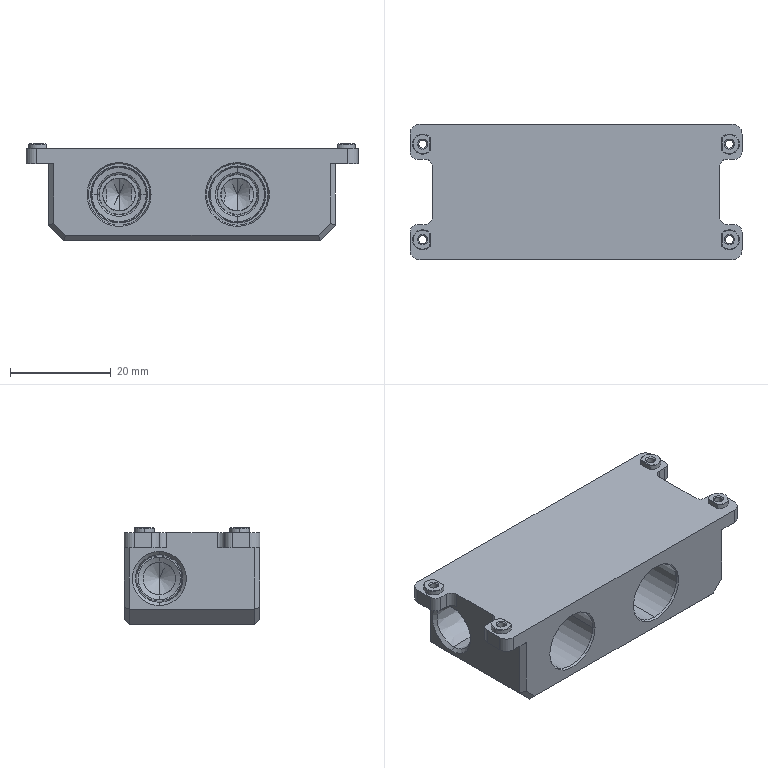NC program | NX | posted with a generic post | part box 66 x 27 x 19.25 mm
Lines 1686 to 2633 of 6448:
(ZLEVEL_PROFILE_STEEP , TOOL : 圆鼻刀)
N3322 T08 M6
N3324 G53
N3326 G17 G0 G90 X-15.95 Y25.719 S6500 M3
N3328 G43 Z20. H8
N3330 Z2.404
N3332 G94 G1 Z1.404 F2000.
N3334 X-15.516 Y25.277
N3336 G3 X-13.819 Y25.262 R1.2
N3338 G2 X-12.468 Y25.803 R1.89
N3340 G1 X12.468
N3342 G2 X13.819 Y25.262 R1.89
N3344 G1 X13.876 Y25.216 Z1.394
N3346 X13.931 Y25.168 Z1.384
N3348 X13.983 Y25.117 Z1.374
N3350 X14.033 Y25.064 Z1.364
N3352 X14.08 Y25.01 Z1.354
N3354 G3 X13.806 Y25.324 R1.983
N3356 G1 X13.759 Y25.367
N3358 G3 X12.496 Y25.853 R1.881
N3360 G1 X-12.509
N3362 G3 X-13.243 Y25.699 R1.818
N3364 X-14.08 Y25.01 R2.008
N3366 G1 X-14.133 Y24.983 Z1.304
N3368 G2 X-13.467 Y25.633 R2.074
N3370 X-12.468 Y25.903 R1.878
N3372 G1 X12.468
N3374 G2 X13.707 Y25.463 R1.896
N3376 X14.133 Y24.983 R2.166
N3378 G1 X14.186 Y24.959 Z1.254
N3380 G3 X13.906 Y25.324 R2.811
N3382 X12.468 Y25.953 R1.909
N3384 G1 X-12.468
N3386 G3 X-13.906 Y25.324 R1.909
N3388 X-14.186 Y24.959 R2.811
N3390 G1 X-14.235 Y24.937 Z1.205
N3392 G2 X-13.951 Y25.324 R4.317
N3394 X-12.468 Y26.003 R1.916
N3396 G1 X12.468
N3398 G2 X13.951 Y25.324 R1.916
N3400 X14.235 Y24.937 R4.318
N3402 G1 X14.286 Y24.916 Z1.155
N3404 X14.017 Y25.294
N3406 X13.964 Y25.358
N3408 G3 X12.485 Y26.052 R1.921
N3410 G1 X-12.485
N3412 G3 X-13.964 Y25.358 R1.921
N3414 G1 X-14.017 Y25.294
N3416 X-14.286 Y24.916
N3418 X-14.337 Y24.895 Z1.105
N3420 X-14.051 Y25.295
N3422 G2 X-12.484 Y26.102 R1.925
N3424 G1 X12.484
N3426 G2 X14.051 Y25.295 R1.925
N3428 G1 X14.337 Y24.895
N3430 X14.387 Y24.874 Z1.055
N3432 X14.052 Y25.344
N3434 G3 X12.485 Y26.152 R1.924
N3436 G1 X-12.485
N3438 G3 X-14.052 Y25.344 R1.924
N3440 G1 X-14.387 Y24.874
N3442 X-14.437 Y24.853 Z1.005
N3444 X-14.052 Y25.394
N3446 G2 X-12.485 Y26.202 R1.923
N3448 G1 X12.485
N3450 G2 X14.052 Y25.394 R1.923
N3452 G1 X14.437 Y24.853
N3454 X14.487 Y24.832 Z0.956
N3456 X14.482 Y24.84
N3458 X14.052 Y25.443
N3460 G3 X12.485 Y26.251 R1.925
N3462 G1 X-12.485
N3464 G3 X-14.052 Y25.443 R1.925
N3466 G1 X-14.482 Y24.84
N3468 X-14.487 Y24.832
N3470 X-14.537 Y24.81 Z0.906
N3472 X-14.503 Y24.86
N3474 X-14.052 Y25.493
N3476 G2 X-12.485 Y26.301 R1.923
N3478 G1 X12.485
N3480 G2 X14.052 Y25.493 R1.923
N3482 G1 X14.503 Y24.86
N3484 X14.537 Y24.81
N3486 X14.587 Y24.789 Z0.856
N3488 X14.538 Y24.86
N3490 X14.053 Y25.542
N3492 G3 X12.485 Y26.351 R1.925
N3494 G1 X-12.485
N3496 G3 X-14.053 Y25.542 R1.925
N3498 G1 X-14.538 Y24.86
N3500 X-14.587 Y24.789
N3502 X-14.638 Y24.768 Z0.806
N3504 G2 X-14.045 Y25.603 R57.54
N3506 X-12.484 Y26.401 R1.927
N3508 G1 X12.484
N3510 G2 X14.045 Y25.603 R1.927
N3512 X14.638 Y24.768 R57.886
N3514 G1 X14.688 Y24.747 Z0.757
N3516 G3 X14.045 Y25.653 R56.973
N3518 X12.483 Y26.451 R1.928
N3520 G1 X-12.483
N3522 G3 X-14.045 Y25.653 R1.928
N3524 X-14.688 Y24.747 R56.616
N3526 G1 X-14.738 Y24.726 Z0.707
N3528 G2 X-14.046 Y25.701 R73.331
N3530 X-12.484 Y26.5 R1.927
N3532 G1 X12.484
N3534 G2 X14.046 Y25.701 R1.927
N3536 X14.738 Y24.725 R73.745
N3538 G1 X14.789 Y24.705 Z0.657
N3540 X14.172 Y25.577
N3542 X14.046 Y25.751
N3544 G3 X12.484 Y26.55 R1.927
N3546 G1 X-12.484
N3548 G3 X-14.046 Y25.751 R1.927
N3550 G1 X-14.172 Y25.577
N3552 X-14.789 Y24.705
N3554 X-14.838 Y24.683 Z0.607
N3556 X-14.824 Y24.705
N3558 X-14.172 Y25.627
N3560 X-14.047 Y25.8
N3562 G2 X-12.483 Y26.6 R1.928
N3564 G1 X12.483
N3566 G2 X14.047 Y25.8 R1.928
N3568 G1 X14.172 Y25.627
N3570 X14.824 Y24.705
N3572 X14.838 Y24.683
N3574 X14.888 Y24.662 Z0.558
N3576 X14.859 Y24.705
N3578 X14.172 Y25.676
N3580 X14.046 Y25.85
N3582 G3 X12.484 Y26.65 R1.927
N3584 G1 X-12.484
N3586 G3 X-14.046 Y25.85 R1.927
N3588 G1 X-14.172 Y25.676
N3590 X-14.859 Y24.705
N3592 X-14.888 Y24.662
N3594 X-14.939 Y24.642 Z0.508
N3596 X-14.894 Y24.705
N3598 X-14.172 Y25.726
N3600 X-14.046 Y25.9
N3602 G2 X-12.484 Y26.699 R1.926
N3604 G1 X12.484
N3606 G2 X14.046 Y25.9 R1.926
N3608 G1 X14.172 Y25.726
N3610 X14.894 Y24.705
N3612 X14.939 Y24.642
N3614 X14.988 Y24.62 Z0.458
N3616 X14.946 Y24.681
N3618 X14.172 Y25.776
N3620 X14.047 Y25.949
N3622 G3 X12.483 Y26.749 R1.929
N3624 G1 X-12.483
N3626 G3 X-14.047 Y25.949 R1.929
N3628 G1 X-14.172 Y25.776
N3630 X-14.946 Y24.681
N3632 X-14.988 Y24.62
N3634 X-15.038 Y24.6 Z0.408
N3636 X-14.964 Y24.705
N3638 X-14.172 Y25.826
N3640 X-14.046 Y26.
N3642 G2 X-12.484 Y26.799 R1.926
N3644 G1 X12.484
N3646 G2 X14.046 Y25.999 R1.926
N3648 G1 X14.172 Y25.826
N3650 X14.964 Y24.705
N3652 X15.038 Y24.6
N3654 X15.088 Y24.579 Z0.358
N3656 X14.172 Y25.875
N3658 X14.042 Y26.055
N3660 G3 X12.486 Y26.849 R1.92
N3662 G1 X-12.486
N3664 G3 X-14.041 Y26.055 R1.92
N3666 G1 X-14.172 Y25.875
N3668 X-15.088 Y24.579
N3670 X-15.138 Y24.559 Z0.309
N3672 X-14.172 Y25.925
N3674 X-14.047 Y26.098
N3676 G2 X-12.483 Y26.898 R1.929
N3678 G1 X12.483
N3680 G2 X14.047 Y26.098 R1.929
N3682 G1 X14.172 Y25.925
N3684 X15.138 Y24.559
N3686 X15.188 Y24.538 Z0.259
N3688 X15.179 Y24.551
N3690 X14.172 Y25.975
N3692 X14.046 Y26.149
N3694 G3 X12.484 Y26.948 R1.926
N3696 G1 X-12.484
N3698 G3 X-14.046 Y26.149 R1.926
N3700 G1 X-14.172 Y25.975
N3702 X-15.179 Y24.551
N3704 X-15.188 Y24.538
N3706 X-15.237 Y24.518 Z0.209
N3708 X-14.172 Y26.025
N3710 X-14.039 Y26.208
N3712 G2 X-12.487 Y26.998 R1.919
N3714 G1 X12.487
N3716 G2 X14.039 Y26.208 R1.919
N3718 G1 X14.172 Y26.025
N3720 X15.237 Y24.518
N3722 X15.286 Y24.497 Z0.159
N3724 X15.256 Y24.542
N3726 X14.172 Y26.074
N3728 X14.046 Y26.249
N3730 G3 X12.485 Y27.048 R1.924
N3732 G1 X-12.485
N3734 G3 X-14.046 Y26.249 R1.924
N3736 G1 X-14.172 Y26.074
N3738 X-15.256 Y24.542
N3740 X-15.286 Y24.497
N3742 X-15.336 Y24.476 Z0.11
N3744 X-15.285 Y24.551
N3746 X-14.172 Y26.124
N3748 X-14.046 Y26.298
N3750 G2 X-12.484 Y27.098 R1.926
N3752 G1 X12.484
N3754 G2 X14.046 Y26.298 R1.926
N3756 G1 X14.172 Y26.124
N3758 X15.285 Y24.551
N3760 X15.336 Y24.476
N3762 X15.386 Y24.456 Z0.06
N3764 X15.32 Y24.551
N3766 X14.172 Y26.174
N3768 X14.047 Y26.347
N3770 G3 X12.483 Y27.147 R1.928
N3772 G1 X-12.483
N3774 G3 X-14.047 Y26.347 R1.928
N3776 G1 X-14.172 Y26.174
N3778 X-15.32 Y24.551
N3780 X-15.386 Y24.456
N3782 X-15.436 Y24.436 Z0.01
N3784 X-15.411 Y24.472
N3786 X-14.172 Y26.224
N3788 X-14.046 Y26.398
N3790 G2 X-12.485 Y27.197 R1.925
N3792 G1 X12.485
N3794 G2 X14.046 Y26.398 R1.925
N3796 G1 X14.172 Y26.224
N3798 X15.411 Y24.472
N3800 X15.436 Y24.436
N3802 X15.485 Y24.416 Z-0.04
N3804 X15.411 Y24.522
N3806 X14.172 Y26.273
N3808 X14.047 Y26.447
N3810 G3 X12.484 Y27.247 R1.927
N3812 G1 X-12.484
N3814 G3 X-14.047 Y26.447 R1.927
N3816 G1 X-14.172 Y26.274
N3818 X-15.411 Y24.522
N3820 X-15.485 Y24.416
N3822 X-15.535 Y24.396 Z-0.09
N3824 X-14.172 Y26.323
N3826 X-14.047 Y26.496
N3828 G2 X-12.483 Y27.297 R1.928
N3830 G1 X12.483
N3832 G2 X14.047 Y26.496 R1.928
N3834 G1 X14.172 Y26.323
N3836 X15.535 Y24.396
N3838 X15.584 Y24.375 Z-0.139
N3840 X15.57 Y24.396
N3842 X14.172 Y26.373
N3844 X14.046 Y26.547
N3846 G3 X12.484 Y27.346 R1.926
N3848 G1 X-12.484
N3850 G3 X-14.046 Y26.547 R1.926
N3852 G1 X-14.172 Y26.373
N3854 X-15.57 Y24.396
N3856 X-15.584 Y24.375
N3858 X-15.633 Y24.355 Z-0.189
N3860 X-15.606 Y24.396
N3862 X-14.172 Y26.423
N3864 X-14.017 Y26.638
N3866 G2 X-12.5 Y27.396 R1.932
N3868 G1 X12.5
N3870 G2 X14.017 Y26.638 R1.932
N3872 G1 X14.172 Y26.423
N3874 X15.606 Y24.396
N3876 X15.634 Y24.355
N3878 X15.683 Y24.334 Z-0.239
N3880 X15.641 Y24.396
N3882 X14.172 Y26.473
N3884 X14.017 Y26.687
N3886 G3 X12.5 Y27.446 R1.928
N3888 G1 X-12.5
N3890 G3 X-14.017 Y26.687 R1.928
N3892 G1 X-14.172 Y26.473
N3894 X-15.641 Y24.396
N3896 X-15.683 Y24.334
N3898 X-15.733 Y24.314 Z-0.289
N3900 X-15.721 Y24.333
N3902 X-14.172 Y26.522
N3904 X-14.034 Y26.716
N3906 G2 X-12.5 Y27.496 R1.933
N3908 G1 X12.5
N3910 G2 X14.034 Y26.716 R1.933
N3912 G1 X14.172 Y26.522
N3914 X15.721 Y24.333
N3916 X15.733 Y24.314
N3918 X15.782 Y24.294 Z-0.338
N3920 X15.721 Y24.383
N3922 X14.07 Y26.716
N3924 G3 X12.5 Y27.545 R1.941
N3926 G1 X-12.5
N3928 G3 X-14.07 Y26.716 R1.941
N3930 G1 X-15.721 Y24.383
N3932 X-15.782 Y24.294
N3934 X-15.832 Y24.274 Z-0.388
N3936 X-15.747 Y24.396
N3938 X-14.216 Y26.559
N3940 X-14.078 Y26.754
N3942 G2 X-12.5 Y27.595 R1.945
N3944 G1 X12.5
N3946 G2 X14.078 Y26.754 R1.945
N3948 G1 X14.216 Y26.559
N3950 X15.747 Y24.396
N3952 X15.832 Y24.274
N3954 X15.882 Y24.254 Z-0.438
N3956 X14.266 Y26.538
N3958 X14.078 Y26.804
N3960 G3 X12.5 Y27.645 R1.945
N3962 G1 X-12.5
N3964 G3 X-14.078 Y26.804 R1.945
N3966 G1 X-14.266 Y26.538
N3968 X-15.882 Y24.254
N3970 X-15.932 Y24.233 Z-0.488
N3972 X-14.316 Y26.518
N3974 X-14.078 Y26.854
N3976 G2 X-12.5 Y27.695 R1.945
N3978 G1 X12.5
N3980 G2 X14.078 Y26.854 R1.945
N3982 G1 X14.316 Y26.518
N3984 X15.932 Y24.233
N3986 X15.981 Y24.213 Z-0.537
N3988 X15.962 Y24.241
N3990 X14.366 Y26.497
N3992 X14.078 Y26.904
N3994 G3 X13.845 Y27.179 R2.184
N3996 X12.5 Y27.745 R1.904
N3998 G1 X-12.512
N4000 G3 X-13.088 Y27.649 R1.786
N4002 X-14.078 Y26.904 R1.989
N4004 G1 X-14.366 Y26.497
N4006 X-15.962 Y24.241
N4008 X-15.981 Y24.213
N4010 X-16.031 Y24.193 Z-0.587
N4012 X-14.416 Y26.476
N4014 X-14.078 Y26.953
N4016 G2 X-13.088 Y27.699 R1.988
N4018 X-12.512 Y27.794 R1.787
N4020 G1 X12.5
N4022 G2 X13.321 Y27.602 R1.846
N4024 X14.078 Y26.953 R2.036
N4026 G1 X14.416 Y26.476
N4028 X16.031 Y24.193
N4030 X16.08 Y24.172 Z-0.637
N4032 X16.032 Y24.241
N4034 X14.465 Y26.456
N4036 X14.078 Y27.003
N4038 G3 X12.5 Y27.844 R1.945
N4040 G1 X-12.5
N4042 G3 X-14.078 Y27.003 R1.945
N4044 G1 X-14.465 Y26.456
N4046 X-16.032 Y24.241
N4048 X-16.08 Y24.172
N4050 X-16.13 Y24.152 Z-0.687
N4052 X-16.067 Y24.241
N4054 X-14.515 Y26.435
N4056 X-14.078 Y27.053
N4058 G2 X-13.088 Y27.799 R1.989
N4060 X-12.512 Y27.894 R1.786
N4062 G1 X12.5
N4064 G2 X13.702 Y27.459 R1.878
N4066 X14.078 Y27.053 R2.16
N4068 G1 X14.515 Y26.435
N4070 X16.067 Y24.241
N4072 X16.13 Y24.152
N4074 X16.18 Y24.132 Z-0.737
N4076 X14.565 Y26.414
N4078 X14.078 Y27.103
N4080 G3 X13.295 Y27.764 R2.03
N4082 X12.5 Y27.944 R1.844
N4084 G1 X-12.512
N4086 G3 X-13.088 Y27.848 R1.788
N4088 X-14.078 Y27.103 R1.988
N4090 G1 X-14.565 Y26.414
N4092 X-16.18 Y24.132
N4094 X-16.229 Y24.111 Z-0.786
N4096 X-16.185 Y24.174
N4098 X-14.615 Y26.394
N4100 X-14.078 Y27.152
N4102 G2 X-12.5 Y27.993 R1.945
N4104 G1 X12.5
N4106 G2 X14.078 Y27.152 R1.945
N4108 G1 X14.615 Y26.394
N4110 X16.185 Y24.174
N4112 X16.229 Y24.111
N4114 X16.279 Y24.091 Z-0.836
N4116 X14.664 Y26.373
N4118 X14.078 Y27.202
N4120 G3 X13.672 Y27.632 R2.138
N4122 X12.5 Y28.043 R1.876
N4124 G1 X-12.509
N4126 G3 X-13.243 Y27.889 R1.819
N4128 X-14.078 Y27.202 R2.009
N4130 G1 X-14.664 Y26.373
N4132 X-16.279 Y24.091
N4134 X-16.328 Y24.071 Z-0.886
N4136 X-16.318 Y24.087
N4138 X-14.714 Y26.353
N4140 X-14.078 Y27.252
N4142 G2 X-13.088 Y27.998 R1.987
N4144 X-12.511 Y28.093 R1.789
N4146 G1 X12.5
N4148 G2 X13.718 Y27.643 R1.893
N4150 X14.078 Y27.252 R2.079
N4152 G1 X14.714 Y26.353
N4154 X16.328 Y24.071
N4156 X16.377 Y24.05 Z-0.936
N4158 X16.353 Y24.087
N4160 X14.764 Y26.332
N4162 X14.078 Y27.302
N4164 G3 X12.5 Y28.143 R1.945
N4166 G1 X-12.5
N4168 G3 X-14.078 Y27.302 R1.945
N4170 G1 X-14.764 Y26.332
N4172 X-16.353 Y24.087
N4174 X-16.377 Y24.05
N4176 X-16.427 Y24.03 Z-0.985
N4178 X-16.388 Y24.087
N4180 X-14.814 Y26.311
N4182 X-14.078 Y27.351
N4184 G2 X-13.243 Y28.038 R2.009
N4186 X-12.509 Y28.193 R1.82
N4188 G1 X12.5
N4190 G2 X13.642 Y27.805 R1.874
N4192 X14.078 Y27.351 R2.119
N4194 G1 X14.814 Y26.311
N4196 X16.388 Y24.087
N4198 X16.427 Y24.03
N4200 X16.477 Y24.01 Z-1.035
N4202 X16.423 Y24.087
N4204 X14.863 Y26.291
N4206 X14.078 Y27.401
N4208 G3 X13.578 Y27.901 R2.084
N4210 X12.5 Y28.242 R1.87
N4212 G1 X-12.511
N4214 G3 X-13.088 Y28.147 R1.79
N4216 X-14.078 Y27.401 R1.986
N4218 G1 X-14.863 Y26.291
N4220 X-16.423 Y24.087
N4222 X-16.477 Y24.01
N4224 X-16.51 Y24.013 Z-1.085
N4226 X-16.495 Y24.035
N4228 X-14.913 Y26.27
N4230 X-14.078 Y27.451
N4232 G2 X-13.088 Y28.197 R1.987
N4234 X-12.511 Y28.292 R1.789
N4236 G1 X12.5
N4238 G2 X13.862 Y27.71 R1.909
N4240 X14.078 Y27.451 R2.225
N4242 G1 X14.913 Y26.27
N4244 X16.495 Y24.035
N4246 X16.51 Y24.013
N4248 X16.523 Y24.021 Z-1.11
N4250 X16.535 Y24.028 Z-1.135
N4252 X16.495 Y24.085
N4254 X14.953 Y26.264
N4256 X14.078 Y27.501
N4258 G3 X13.613 Y27.975 R2.104
N4260 X12.5 Y28.342 R1.872
N4262 G1 X-12.512
N4264 G3 X-13.088 Y28.246 R1.787
N4266 X-14.078 Y27.501 R1.988
N4268 G1 X-14.953 Y26.264
N4270 X-16.495 Y24.085
N4272 X-16.535 Y24.028
N4274 X-16.547 Y24.036 Z-1.16
N4276 X-16.559 Y24.044 Z-1.185
N4278 X-14.973 Y26.286
N4280 X-14.078 Y27.551
N4282 G2 X-13.088 Y28.296 R1.986
N4284 X-12.511 Y28.392 R1.792
N4286 G1 X12.5
N4288 G2 X13.699 Y27.96 R1.878
N4290 X14.078 Y27.551 R2.143
N4292 G1 X14.973 Y26.286
N4294 X16.559 Y24.044
N4296 X16.571 Y24.051 Z-1.209
N4298 X16.584 Y24.059 Z-1.234
N4300 X14.992 Y26.308
N4302 X14.078 Y27.6
N4304 G3 X13.862 Y27.859 R2.25
N4306 X12.5 Y28.441 R1.909
N4308 G1 X-12.511
N4310 G3 X-13.088 Y28.346 R1.788
N4312 X-14.078 Y27.6 R1.988
N4314 G1 X-14.992 Y26.308
N4316 X-16.583 Y24.059
N4318 X-16.596 Y24.067 Z-1.259
N4320 X-16.608 Y24.075 Z-1.284
N4322 X-15.012 Y26.33
N4324 X-14.078 Y27.65
N4326 G2 X-13.088 Y28.396 R1.987
N4328 X-12.511 Y28.491 R1.789
N4330 G1 X12.5
N4332 G2 X13.591 Y28.14 R1.871
N4334 X14.078 Y27.65 R2.092
N4336 G1 X15.012 Y26.33
N4338 X16.608 Y24.075
N4340 X16.627 Y24.097 Z-1.334
N4342 X15.078 Y26.286
N4344 X14.078 Y27.7
N4346 G3 X12.5 Y28.541 R1.945
N4348 G1 X-12.5
N4350 G3 X-14.078 Y27.7 R1.945
N4352 G1 X-15.078 Y26.286
N4354 X-16.627 Y24.097
N4356 Y24.147 Z-1.384
N4358 X-16.56 Y24.241
N4360 X-15.078 Y26.335
N4362 X-14.078 Y27.75
N4364 G2 X-13.088 Y28.495 R1.988
N4366 X-12.511 Y28.591 R1.788
N4368 G1 X12.5
N4370 G2 X13.482 Y28.311 R1.861
N4372 X14.078 Y27.75 R2.068
N4374 G1 X15.078 Y26.335
N4376 X16.56 Y24.241
N4378 X16.627 Y24.147
N4380 Y24.196 Z-1.433
N4382 X16.596 Y24.241
N4384 X15.078 Y26.385
N4386 X14.078 Y27.799
N4388 G3 X13.574 Y28.302 R2.083
N4390 X12.5 Y28.64 R1.871
N4392 G1 X-12.511
N4394 G3 X-13.088 Y28.545 R1.79
N4396 X-14.078 Y27.799 R1.987
N4398 G1 X-15.078 Y26.385
N4400 X-16.596 Y24.241
N4402 X-16.627 Y24.196
N4404 Y24.246 Z-1.483
N4406 X-15.078 Y26.435
N4408 X-14.078 Y27.849
N4410 G2 X-12.5 Y28.69 R1.945
N4412 G1 X12.5
N4414 G2 X14.078 Y27.849 R1.945
N4416 G1 X15.078 Y26.435
N4418 X16.628 Y24.246
N4420 Y24.295 Z-1.533
N4422 X16.557 Y24.396
N4424 X15.078 Y26.485
N4426 X14.078 Y27.899
N4428 G3 X13.438 Y28.486 R2.059
N4430 X12.5 Y28.74 R1.857
N4432 G1 X-12.511
N4434 G3 X-13.088 Y28.645 R1.789
N4436 X-14.078 Y27.899 R1.987
N4438 G1 X-15.078 Y26.485
N4440 X-16.557 Y24.396
N4442 X-16.627 Y24.295
N4444 X-16.628 Y24.345 Z-1.583
N4446 X-16.592 Y24.396
N4448 X-15.078 Y26.534
N4450 X-14.078 Y27.949
N4452 G2 X-13.088 Y28.694 R1.987
N4454 X-12.511 Y28.79 R1.789
N4456 G1 X12.5
N4458 G2 X13.862 Y28.208 R1.909
N4460 X14.078 Y27.949 R2.206
N4462 G1 X15.078 Y26.534
N4464 X16.592 Y24.396
N4466 X16.628 Y24.345
N4468 Y24.394 Z-1.632
N4470 X15.078 Y26.584
N4472 X14.078 Y27.998
N4474 G3 X12.5 Y28.84 R1.945
N4476 G1 X-12.5
N4478 G3 X-14.078 Y27.998 R1.945
N4480 G1 X-15.078 Y26.584
N4482 X-16.628 Y24.394
N4484 Y24.444 Z-1.682
N4486 X-16.553 Y24.551
N4488 X-15.078 Y26.634
N4490 X-14.078 Y28.048
N4492 G2 X-13.088 Y28.794 R1.988
N4494 X-12.512 Y28.889 R1.787
N4496 G1 X12.5
N4498 G2 X13.862 Y28.307 R1.909
N4500 G1 X13.904 Y28.262
N4502 G2 X14.078 Y28.048 R2.051
N4504 G1 X15.078 Y26.634
N4506 X16.553 Y24.551
N4508 X16.628 Y24.444
N4510 Y24.493 Z-1.732
N4512 X16.588 Y24.551
N4514 X15.078 Y26.684
N4516 X14.078 Y28.098
N4518 G3 X13.862 Y28.357 R2.179
N4520 X12.5 Y28.939 R1.909
N4522 G1 X-12.511
N4524 G3 X-13.088 Y28.844 R1.789
N4526 X-14.078 Y28.098 R1.987
N4528 G1 X-15.078 Y26.684
N4530 X-16.588 Y24.551
N4532 X-16.628 Y24.493
N4534 X-16.629 Y24.543 Z-1.782
N4536 X-15.078 Y26.734
N4538 X-14.078 Y28.148
N4540 G2 X-13.088 Y28.894 R1.988
N4542 X-12.511 Y28.989 R1.788
N4544 G1 X12.5
N4546 G2 X13.852 Y28.417 R1.906
N4548 X14.078 Y28.148 R2.218
N4550 G1 X15.078 Y26.734
N4552 X16.629 Y24.543
N4554 Y24.592 Z-1.832
N4556 X16.549 Y24.705
N4558 X15.078 Y26.783
N4560 X14.078 Y28.198
N4562 G3 X13.361 Y28.826 R2.044
N4564 X12.5 Y29.039 R1.849
N4566 G1 X-12.512
N4568 G3 X-13.088 Y28.943 R1.787
N4570 X-14.078 Y28.198 R1.988
N4572 G1 X-15.078 Y26.783
N4574 X-16.549 Y24.705
N4576 X-16.629 Y24.592
N4578 Y24.642 Z-1.881
N4580 X-16.584 Y24.705
N4582 X-15.078 Y26.833
N4584 X-14.078 Y28.247
N4586 G2 X-12.5 Y29.088 R1.945
N4588 G1 X12.5
N4590 G2 X14.078 Y28.247 R1.945
N4592 G1 X15.078 Y26.833
N4594 X16.584 Y24.705
N4596 X16.629 Y24.642
N4598 Y24.691 Z-1.931
N4600 X15.078 Y26.883
N4602 X14.078 Y28.297
N4604 G3 X13.847 Y28.571 R2.193
N4606 X12.5 Y29.138 R1.904
N4608 G1 X-12.512
N4610 G3 X-13.088 Y29.043 R1.787
N4612 X-14.078 Y28.297 R1.989
N4614 G1 X-15.078 Y26.883
N4616 X-16.629 Y24.691
N4618 Y24.741 Z-1.981
N4620 X-16.545 Y24.86
N4622 X-15.078 Y26.933
N4624 X-14.078 Y28.347
N4626 G2 X-13.088 Y29.093 R1.988
N4628 X-12.512 Y29.188 R1.787
N4630 G1 X12.5
N4632 G2 X13.33 Y28.991 R1.846
N4634 X14.078 Y28.347 R2.038
N4636 G1 X15.078 Y26.933
N4638 X16.545 Y24.86
N4640 X16.629 Y24.741
N4642 Y24.79 Z-2.031
N4644 X15.078 Y26.982
N4646 X14.078 Y28.397
N4648 G3 X12.5 Y29.238 R1.945
N4650 G1 X-12.5
N4652 G3 X-14.078 Y28.397 R1.945
N4654 G1 X-15.078 Y26.982
N4656 X-16.629 Y24.79
N4658 X-16.63 Y24.84 Z-2.08
N4660 X-15.078 Y27.032
N4662 X-14.078 Y28.446
N4664 G2 X-13.088 Y29.192 R1.989
N4666 X-12.512 Y29.288 R1.786
N4668 G1 X12.5
N4670 G2 X13.712 Y28.844 R1.878
N4672 X14.078 Y28.446 R2.168
N4674 G1 X15.078 Y27.032
N4676 X16.63 Y24.84
N4678 Y24.889 Z-2.13
N4680 X16.542 Y25.015
N4682 X15.078 Y27.082
N4684 X14.078 Y28.496
N4686 G3 X13.302 Y29.154 R2.032
N4688 X12.5 Y29.337 R1.844
N4690 G1 X-12.512
N4692 G3 X-13.088 Y29.242 R1.787
N4694 X-14.078 Y28.496 R1.988
N4696 G1 X-15.078 Y27.082
N4698 X-16.542 Y25.015
N4700 X-16.63 Y24.889
N4702 Y24.939 Z-2.18
N4704 X-15.078 Y27.132
N4706 X-14.078 Y28.546
N4708 G2 X-12.5 Y29.387 R1.945
N4710 G1 X12.5
N4712 G2 X14.078 Y28.546 R1.945
N4714 G1 X15.078 Y27.132
N4716 X16.63 Y24.939
N4718 Y24.988 Z-2.23
N4720 X15.078 Y27.182
N4722 X14.078 Y28.596
N4724 G3 X13.683 Y29.017 R2.145
N4726 X12.5 Y29.437 R1.876
N4728 G1 X-12.512
N4730 G3 X-13.088 Y29.341 R1.786
N4732 X-14.078 Y28.596 R1.989
N4734 G1 X-15.078 Y27.182
N4736 X-16.63 Y24.988
N4738 Y25.038 Z-2.279
N4740 X-15.078 Y27.231
N4742 X-14.078 Y28.646
N4744 G2 X-13.088 Y29.391 R1.988
N4746 X-12.511 Y29.487 R1.788
N4748 G1 X12.5
N4750 G2 X13.279 Y29.314 R1.842
N4752 X14.078 Y28.646 R2.027
N4754 G1 X15.078 Y27.231
N4756 X16.63 Y25.038
N4758 X16.631 Y25.087 Z-2.329
N4760 X15.078 Y27.281
N4762 X14.078 Y28.695
N4764 G3 X12.5 Y29.536 R1.945
N4766 G1 X-12.5
N4768 G3 X-14.078 Y28.695 R1.945
N4770 G1 X-15.078 Y27.281
N4772 X-16.631 Y25.087
N4774 Y25.137 Z-2.379
N4776 X-15.078 Y27.331
N4778 X-14.078 Y28.745
N4780 G2 X-13.243 Y29.432 R2.009
N4782 X-12.509 Y29.586 R1.82
N4784 G1 X12.5
N4786 G2 X13.707 Y29.146 R1.895
N4788 G1 X13.79 Y29.071
N4790 G2 X14.074 Y28.751 R1.952
N4792 G1 X15.078 Y27.331
N4794 X16.631 Y25.137
N4796 Y25.186 Z-2.429
N4798 X15.078 Y27.381
N4800 X14.078 Y28.795
N4802 G3 X13.502 Y29.344 R2.063
N4804 X12.5 Y29.636 R1.865
N4806 G1 X-12.511
N4808 G3 X-13.088 Y29.541 R1.79
N4810 X-14.078 Y28.795 R1.987
N4812 G1 X-15.078 Y27.381
N4814 X-16.631 Y25.187
N4816 Y25.236 Z-2.479
N4818 X-15.078 Y27.43
N4820 X-14.078 Y28.845
N4822 G2 X-12.5 Y29.686 R1.945
N4824 G1 X12.5
N4826 G2 X14.078 Y28.845 R1.945
N4828 G1 X15.078 Y27.43
N4830 X16.631 Y25.236
N4832 Y25.285 Z-2.528
N4834 X15.078 Y27.48
N4836 X14.078 Y28.894
N4838 G3 X13.624 Y29.361 R2.109
N4840 X12.5 Y29.735 R1.873
N4842 G1 X-12.512
N4844 G3 X-13.088 Y29.64 R1.787
N4846 X-14.078 Y28.894 R1.989
N4848 G1 X-15.078 Y27.48
N4850 X-16.631 Y25.286
N4852 X-16.632 Y25.335 Z-2.578
N4854 X-15.078 Y27.53
N4856 X-14.078 Y28.944
N4858 G2 X-13.088 Y29.69 R1.986
N4860 X-12.511 Y29.785 R1.792
N4862 G1 X12.5
N4864 G2 X13.666 Y29.379 R1.876
N4866 X14.078 Y28.944 R2.123
N4868 G1 X15.078 Y27.53
N4870 X16.632 Y25.335
N4872 Y25.384 Z-2.628
N4874 X15.078 Y27.58
N4876 X14.078 Y28.994
N4878 G3 X13.862 Y29.253 R2.242
N4880 X12.5 Y29.835 R1.909
N4882 G1 X-12.511
N4884 G3 X-13.088 Y29.74 R1.788
N4886 X-14.078 Y28.994 R1.988
N4888 G1 X-15.078 Y27.58
N4890 X-16.632 Y25.384
N4892 Y25.434 Z-2.678
N4894 X-15.078 Y27.629
N4896 X-14.078 Y29.044
N4898 G2 X-13.088 Y29.789 R1.988
N4900 X-12.511 Y29.885 R1.788
N4902 G1 X12.5
N4904 G2 X13.597 Y29.53 R1.871
N4906 X14.078 Y29.044 R2.096
N4908 G1 X15.078 Y27.629
N4910 X16.632 Y25.434
N4912 Y25.484 Z-2.727
N4914 X15.078 Y27.679
N4916 X14.078 Y29.093
N4918 G3 X12.5 Y29.935 R1.945
N4920 G1 X-12.5
N4922 G3 X-14.078 Y29.093 R1.945
N4924 G1 X-15.078 Y27.679
N4926 X-16.632 Y25.484
N4928 Y25.533 Z-2.777
N4930 X-15.078 Y27.729
N4932 X-14.078 Y29.143
N4934 G2 X-13.088 Y29.889 R1.988
N4936 X-12.511 Y29.984 R1.788
N4938 G1 X12.5
N4940 G2 X13.862 Y29.402 R1.909
N4942 X14.078 Y29.143 R2.261
N4944 G1 X15.078 Y27.729
N4946 X16.632 Y25.533
N4948 Y25.583 Z-2.827
N4950 X15.078 Y27.779
N4952 X14.078 Y29.193
N4954 G3 X13.579 Y29.692 R2.086
N4956 X12.5 Y30.034 R1.871
N4958 G1 X-12.511
N4960 G3 X-13.088 Y29.939 R1.789
N4962 X-14.078 Y29.193 R1.987
N4964 G1 X-15.078 Y27.779
N4966 X-16.632 Y25.583
N4968 X-16.633 Y25.632 Z-2.877
N4970 X-15.078 Y27.829
N4972 X-14.078 Y29.243
N4974 G2 X-12.5 Y30.084 R1.945
N4976 G1 X12.5
N4978 G2 X14.078 Y29.243 R1.945
N4980 G1 X15.078 Y27.829
N4982 X16.633 Y25.632
N4984 Y25.682 Z-2.927
N4986 X15.078 Y27.878
N4988 X14.078 Y29.293
N4990 G3 X13.453 Y29.871 R2.062
N4992 X12.5 Y30.134 R1.858
N4994 G1 X-12.511
N4996 G3 X-13.088 Y30.038 R1.789
N4998 X-14.078 Y29.293 R1.987
N5000 G1 X-15.078 Y27.878
N5002 X-16.633 Y25.682
N5004 Y25.731 Z-2.976
N5006 X-15.078 Y27.928
N5008 X-14.078 Y29.342
N5010 G2 X-13.088 Y30.088 R1.988
N5012 X-12.512 Y30.183 R1.788
N5014 G1 X12.5
N5016 G2 X13.565 Y29.85 R1.87
N5018 X14.078 Y29.342 R2.078
N5020 G1 X15.078 Y27.928
N5022 X16.633 Y25.731
N5024 Y25.781 Z-3.026
N5026 X15.078 Y27.978
N5028 X14.078 Y29.392
N5030 G3 X12.5 Y30.233 R1.945
N5032 G1 X-12.5
N5034 G3 X-14.078 Y29.392 R1.945
N5036 G1 X-15.078 Y27.978
N5038 X-16.633 Y25.781
N5040 Y25.831 Z-3.076
N5042 X-15.078 Y28.028
N5044 X-14.078 Y29.442
N5046 G2 X-13.088 Y30.188 R1.991
N5048 X-12.512 Y30.283 R1.783
N5050 G1 X12.5
N5052 G2 X13.395 Y30.052 R1.853
N5054 X14.078 Y29.442 R2.051
N5056 G1 X15.078 Y28.028
N5058 X16.633 Y25.831
N5060 Y25.88 Z-3.126
N5062 X15.078 Y28.077
N5064 X14.078 Y29.492
N5066 G3 X13.836 Y29.777 R2.147
N5068 X12.479 Y30.333 R1.932
N5070 G1 X-12.514
N5072 G3 X-12.933 Y30.282 R1.739
N5074 X-14.078 Y29.492 R1.972
N5076 G1 X-15.078 Y28.077
N5078 X-16.633 Y25.88
N5080 Y25.93 Z-3.175
N5082 X-15.078 Y28.127
N5084 X-14.078 Y29.541
N5086 G2 X-13.088 Y30.287 R1.986
N5088 X-12.511 Y30.382 R1.791
N5090 G1 X12.481
N5092 G2 X13.862 Y29.801 R1.909
N5094 X14.078 Y29.541 R2.327
N5096 G1 X15.078 Y28.127
N5098 X16.633 Y25.93
N5100 Y25.979 Z-3.225
N5102 X15.078 Y28.177
N5104 X14.078 Y29.591
N5106 G3 X13.901 Y29.808 R2.015
N5108 G1 X13.887 Y29.823
N5110 G3 X12.49 Y30.432 R1.908
N5112 G1 X-12.512
N5114 G3 X-13.088 Y30.337 R1.788
N5116 X-14.078 Y29.591 R1.988
N5118 G1 X-15.078 Y28.177
N5120 X-16.633 Y25.98
N5122 Y26.029 Z-3.275
N5124 X-15.078 Y28.227
N5126 X-14.081 Y29.638
N5128 G2 X-13.709 Y30.041 R2.124
N5130 X-12.468 Y30.482 R1.896
N5132 G1 X12.468
N5134 G2 X13.867 Y29.895 R1.909
N5136 X14.088 Y29.628 R2.32
N5138 G1 X15.078 Y28.227
N5140 X16.633 Y26.029
N5142 X16.634 Y26.079 Z-3.325
N5144 X15.078 Y28.276
N5146 X14.259 Y29.436
N5148 X14.017 Y29.773
N5150 X13.963 Y29.838
N5152 G3 X12.486 Y30.532 R1.92
N5154 G1 X-12.486
N5156 G3 X-13.963 Y29.838 R1.92
N5158 G1 X-14.017 Y29.773
N5160 X-14.259 Y29.436
N5162 X-15.078 Y28.276
N5164 X-16.634 Y26.079
N5166 Y26.129 Z-3.374
N5168 X-15.078 Y28.326
N5170 X-14.379 Y29.316
N5172 X-14.052 Y29.774
N5174 G2 X-12.484 Y30.582 R1.925
N5176 G1 X12.484
N5178 G2 X14.052 Y29.774 R1.925
N5180 G1 X14.379 Y29.316
N5182 X15.078 Y28.326
N5184 X16.634 Y26.129
N5186 Y26.178 Z-3.424
N5188 X15.078 Y28.376
N5190 X14.499 Y29.195
N5192 X14.052 Y29.823
N5194 G3 X12.485 Y30.631 R1.923
N5196 G1 X-12.485
N5198 G3 X-14.052 Y29.823 R1.923
N5200 G1 X-14.499 Y29.195
N5202 X-15.078 Y28.376
N5204 X-16.634 Y26.178
N5206 Y26.228 Z-3.474
N5208 X-15.078 Y28.426
N5210 X-14.172 Y29.708